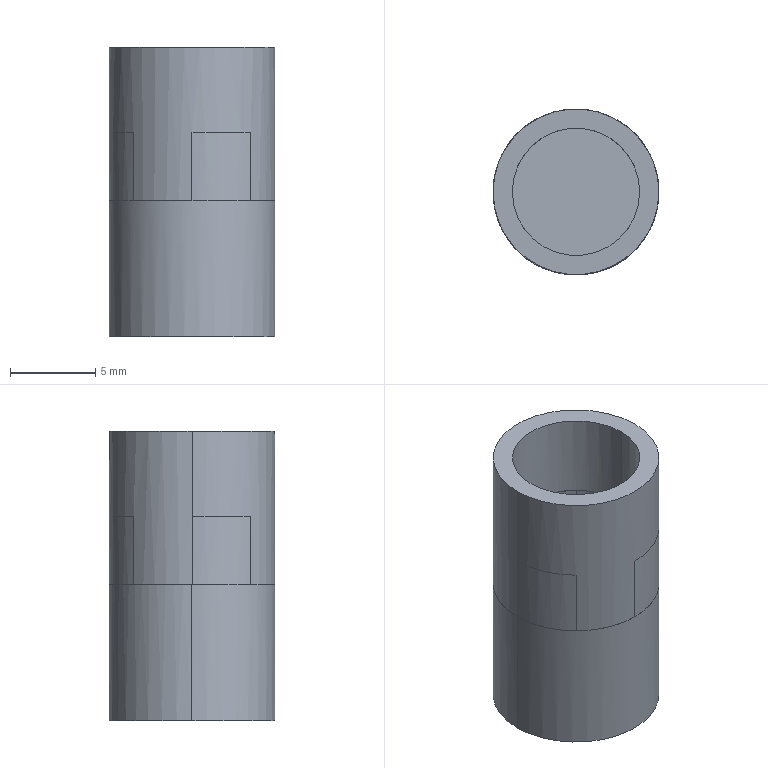Part | SolidWorks | features ICE 3, Extrusion 1 | 2 solids | 47 faces | box 9.746 x 9.746 x 17 mm | volume 515.173 mm3 | plane 28 | cylinder 19 | commonest cylinder face diameters 9.73 x6 7.5 x5 7.516 x4 7.484 x2 9.746 x2
STEP:
#1=CARTESIAN_POINT('',(-3.75,0.007782,-4.));
#2=VERTEX_POINT('',#1);
#3=CARTESIAN_POINT('',(3.75,0.007782,-4.));
#4=VERTEX_POINT('',#3);
#5=CARTESIAN_POINT('',(0.000001501,0.007782,-4.));
#6=DIRECTION('',(0.,0.,1.));
#7=DIRECTION('',(1.,0.,0.));
#8=AXIS2_PLACEMENT_3D('',#5,#6,#7);
#9=CIRCLE('',#8,3.75);
#10=EDGE_CURVE('',#2,#4,#9,.T.);
#11=ORIENTED_EDGE('',*,*,#10,.F.);
#12=CARTESIAN_POINT('',(-3.75,0.007782,4.));
#13=VERTEX_POINT('',#12);
#14=CARTESIAN_POINT('',(-3.75,0.007782,-4.));
#15=DIRECTION('',(0.,0.,1.));
#16=VECTOR('',#15,1000.);
#17=LINE('',#14,#16);
#18=EDGE_CURVE('',#2,#13,#17,.T.);
#19=ORIENTED_EDGE('',*,*,#18,.T.);
#20=CARTESIAN_POINT('',(3.75,0.007782,4.));
#21=VERTEX_POINT('',#20);
#22=CARTESIAN_POINT('',(0.000001501,0.007782,4.));
#23=DIRECTION('',(0.,0.,1.));
#24=DIRECTION('',(1.,0.,0.));
#25=AXIS2_PLACEMENT_3D('',#22,#23,#24);
#26=CIRCLE('',#25,3.75);
#27=EDGE_CURVE('',#13,#21,#26,.T.);
#28=ORIENTED_EDGE('',*,*,#27,.T.);
#29=CARTESIAN_POINT('',(3.75,0.007782,-4.));
#30=DIRECTION('',(0.,0.,1.));
#31=VECTOR('',#30,1000.);
#32=LINE('',#29,#31);
#33=EDGE_CURVE('',#4,#21,#32,.T.);
#34=ORIENTED_EDGE('',*,*,#33,.F.);
#35=EDGE_LOOP('',(#11,#19,#28,#34));
#36=FACE_OUTER_BOUND('',#35,.T.);
#37=CARTESIAN_POINT('',(0.000001501,0.007782,-4.));
#38=DIRECTION('',(0.,0.,1.));
#39=DIRECTION('',(1.,0.,0.));
#40=AXIS2_PLACEMENT_3D('',#37,#38,#39);
#41=CYLINDRICAL_SURFACE('',#40,3.75);
#42=ADVANCED_FACE('',(#36),#41,.F.);
#43=CARTESIAN_POINT('',(4.873,0.007782,-4.));
#44=VERTEX_POINT('',#43);
#45=CARTESIAN_POINT('',(-4.873,0.007782,-4.));
#46=VERTEX_POINT('',#45);
#47=CARTESIAN_POINT('',(0.000001501,0.007782,-4.));
#48=DIRECTION('',(0.,0.,1.));
#49=DIRECTION('',(1.,0.,0.));
#50=AXIS2_PLACEMENT_3D('',#47,#48,#49);
#51=CIRCLE('',#50,4.873);
#52=EDGE_CURVE('',#44,#46,#51,.T.);
#53=ORIENTED_EDGE('',*,*,#52,.T.);
#54=CARTESIAN_POINT('',(-4.873,0.007782,4.));
#55=VERTEX_POINT('',#54);
#56=CARTESIAN_POINT('',(-4.873,0.007782,-4.));
#57=DIRECTION('',(0.,0.,1.));
#58=VECTOR('',#57,1000.);
#59=LINE('',#56,#58);
#60=EDGE_CURVE('',#46,#55,#59,.T.);
#61=ORIENTED_EDGE('',*,*,#60,.T.);
#62=CARTESIAN_POINT('',(4.873,0.007782,4.));
#63=VERTEX_POINT('',#62);
#64=CARTESIAN_POINT('',(0.000001501,0.007782,4.));
#65=DIRECTION('',(0.,0.,1.));
#66=DIRECTION('',(1.,0.,0.));
#67=AXIS2_PLACEMENT_3D('',#64,#65,#66);
#68=CIRCLE('',#67,4.873);
#69=EDGE_CURVE('',#63,#55,#68,.T.);
#70=ORIENTED_EDGE('',*,*,#69,.F.);
#71=CARTESIAN_POINT('',(4.873,0.007782,-4.));
#72=DIRECTION('',(0.,0.,1.));
#73=VECTOR('',#72,1000.);
#74=LINE('',#71,#73);
#75=EDGE_CURVE('',#44,#63,#74,.T.);
#76=ORIENTED_EDGE('',*,*,#75,.F.);
#77=EDGE_LOOP('',(#53,#61,#70,#76));
#78=FACE_OUTER_BOUND('',#77,.T.);
#79=CARTESIAN_POINT('',(0.000001501,0.007782,-4.));
#80=DIRECTION('',(0.,0.,1.));
#81=DIRECTION('',(1.,0.,0.));
#82=AXIS2_PLACEMENT_3D('',#79,#80,#81);
#83=CYLINDRICAL_SURFACE('',#82,4.873);
#84=ADVANCED_FACE('',(#78),#83,.T.);
#85=CARTESIAN_POINT('',(3.758,0.,4.));
#86=VERTEX_POINT('',#85);
#87=CARTESIAN_POINT('',(4.865,0.,4.));
#88=VERTEX_POINT('',#87);
#89=CARTESIAN_POINT('',(3.758,0.,4.));
#90=DIRECTION('',(1.,0.,0.));
#91=VECTOR('',#90,1000.);
#92=LINE('',#89,#91);
#93=EDGE_CURVE('',#86,#88,#92,.T.);
#94=ORIENTED_EDGE('',*,*,#93,.F.);
#95=CARTESIAN_POINT('',(2.656,2.655,4.));
#96=VERTEX_POINT('',#95);
#97=CARTESIAN_POINT('',(0.007782,-0.000001501,4.));
#98=DIRECTION('',(0.,0.,1.));
#99=DIRECTION('',(1.,0.,0.));
#100=AXIS2_PLACEMENT_3D('',#97,#98,#99);
#101=CIRCLE('',#100,3.75);
#102=EDGE_CURVE('',#86,#96,#101,.T.);
#103=ORIENTED_EDGE('',*,*,#102,.T.);
#104=CARTESIAN_POINT('',(0.000001501,0.007782,4.));
#105=DIRECTION('',(0.,0.,1.));
#106=DIRECTION('',(1.,0.,0.));
#107=AXIS2_PLACEMENT_3D('',#104,#105,#106);
#108=CIRCLE('',#107,3.75);
#109=EDGE_CURVE('',#21,#96,#108,.T.);
#110=ORIENTED_EDGE('',*,*,#109,.F.);
#111=ORIENTED_EDGE('',*,*,#27,.F.);
#112=CARTESIAN_POINT('',(-2.656,2.656,4.));
#113=VERTEX_POINT('',#112);
#114=CARTESIAN_POINT('',(0.000001501,0.007782,4.));
#115=DIRECTION('',(0.,0.,1.));
#116=DIRECTION('',(1.,0.,0.));
#117=AXIS2_PLACEMENT_3D('',#114,#115,#116);
#118=CIRCLE('',#117,3.75);
#119=EDGE_CURVE('',#113,#13,#118,.T.);
#120=ORIENTED_EDGE('',*,*,#119,.F.);
#121=CARTESIAN_POINT('',(-3.44,3.44,4.));
#122=VERTEX_POINT('',#121);
#123=CARTESIAN_POINT('',(-2.656,2.656,4.));
#124=DIRECTION('',(0.7071,-0.7071,0.));
#125=VECTOR('',#124,1000.);
#126=LINE('',#123,#125);
#127=EDGE_CURVE('',#122,#113,#126,.T.);
#128=ORIENTED_EDGE('',*,*,#127,.F.);
#129=CARTESIAN_POINT('',(0.,4.865,4.));
#130=VERTEX_POINT('',#129);
#131=CARTESIAN_POINT('',(0.,0.,4.));
#132=DIRECTION('',(0.,0.,1.));
#133=DIRECTION('',(1.,0.,0.));
#134=AXIS2_PLACEMENT_3D('',#131,#132,#133);
#135=CIRCLE('',#134,4.865);
#136=EDGE_CURVE('',#130,#122,#135,.T.);
#137=ORIENTED_EDGE('',*,*,#136,.F.);
#138=CARTESIAN_POINT('',(0.,3.758,4.));
#139=VERTEX_POINT('',#138);
#140=CARTESIAN_POINT('',(0.,3.758,4.));
#141=DIRECTION('',(0.,1.,0.));
#142=VECTOR('',#141,1000.);
#143=LINE('',#140,#142);
#144=EDGE_CURVE('',#139,#130,#143,.T.);
#145=ORIENTED_EDGE('',*,*,#144,.F.);
#146=CARTESIAN_POINT('',(2.656,2.656,4.));
#147=VERTEX_POINT('',#146);
#148=CARTESIAN_POINT('',(0.000001501,0.007782,4.));
#149=DIRECTION('',(0.,0.,1.));
#150=DIRECTION('',(1.,0.,0.));
#151=AXIS2_PLACEMENT_3D('',#148,#149,#150);
#152=CIRCLE('',#151,3.75);
#153=EDGE_CURVE('',#147,#139,#152,.T.);
#154=ORIENTED_EDGE('',*,*,#153,.F.);
#155=CARTESIAN_POINT('',(3.44,3.44,4.));
#156=VERTEX_POINT('',#155);
#157=CARTESIAN_POINT('',(2.656,2.656,4.));
#158=DIRECTION('',(-0.7071,-0.7071,0.));
#159=VECTOR('',#158,1000.);
#160=LINE('',#157,#159);
#161=EDGE_CURVE('',#156,#147,#160,.T.);
#162=ORIENTED_EDGE('',*,*,#161,.F.);
#163=CARTESIAN_POINT('',(0.,0.,4.));
#164=DIRECTION('',(0.,0.,1.));
#165=DIRECTION('',(1.,0.,0.));
#166=AXIS2_PLACEMENT_3D('',#163,#164,#165);
#167=CIRCLE('',#166,4.865);
#168=EDGE_CURVE('',#88,#156,#167,.T.);
#169=ORIENTED_EDGE('',*,*,#168,.F.);
#170=EDGE_LOOP('',(#94,#103,#110,#111,#120,#128,#137,#145,#154,#162,#169));
#171=FACE_BOUND('',#170,.T.);
#172=CARTESIAN_POINT('',(0.,-3.758,4.));
#173=VERTEX_POINT('',#172);
#174=CARTESIAN_POINT('',(0.,-4.865,4.));
#175=VERTEX_POINT('',#174);
#176=CARTESIAN_POINT('',(0.,-3.758,4.));
#177=DIRECTION('',(0.,-1.,0.));
#178=VECTOR('',#177,1000.);
#179=LINE('',#176,#178);
#180=EDGE_CURVE('',#173,#175,#179,.T.);
#181=ORIENTED_EDGE('',*,*,#180,.F.);
#182=CARTESIAN_POINT('',(2.656,-2.656,4.));
#183=VERTEX_POINT('',#182);
#184=CARTESIAN_POINT('',(-0.000001501,-0.007782,4.));
#185=DIRECTION('',(0.,0.,-1.));
#186=DIRECTION('',(1.,0.,0.));
#187=AXIS2_PLACEMENT_3D('',#184,#185,#186);
#188=CIRCLE('',#187,3.75);
#189=EDGE_CURVE('',#183,#173,#188,.T.);
#190=ORIENTED_EDGE('',*,*,#189,.F.);
#191=CARTESIAN_POINT('',(3.44,-3.44,4.));
#192=VERTEX_POINT('',#191);
#193=CARTESIAN_POINT('',(2.656,-2.656,4.));
#194=DIRECTION('',(-0.7071,0.7071,0.));
#195=VECTOR('',#194,1000.);
#196=LINE('',#193,#195);
#197=EDGE_CURVE('',#192,#183,#196,.T.);
#198=ORIENTED_EDGE('',*,*,#197,.F.);
#199=CARTESIAN_POINT('',(0.,0.,4.));
#200=DIRECTION('',(0.,0.,1.));
#201=DIRECTION('',(1.,0.,0.));
#202=AXIS2_PLACEMENT_3D('',#199,#200,#201);
#203=CIRCLE('',#202,4.865);
#204=EDGE_CURVE('',#175,#192,#203,.T.);
#205=ORIENTED_EDGE('',*,*,#204,.F.);
#206=CARTESIAN_POINT('',(0.000001501,0.007782,4.));
#207=DIRECTION('',(0.,0.,1.));
#208=DIRECTION('',(1.,0.,0.));
#209=AXIS2_PLACEMENT_3D('',#206,#207,#208);
#210=CIRCLE('',#209,4.873);
#211=EDGE_CURVE('',#175,#63,#210,.T.);
#212=ORIENTED_EDGE('',*,*,#211,.T.);
#213=ORIENTED_EDGE('',*,*,#69,.T.);
#214=CARTESIAN_POINT('',(0.000001501,0.007782,4.));
#215=DIRECTION('',(0.,0.,1.));
#216=DIRECTION('',(1.,0.,0.));
#217=AXIS2_PLACEMENT_3D('',#214,#215,#216);
#218=CIRCLE('',#217,4.873);
#219=EDGE_CURVE('',#55,#175,#218,.T.);
#220=ORIENTED_EDGE('',*,*,#219,.T.);
#221=EDGE_LOOP('',(#181,#190,#198,#205,#212,#213,#220));
#222=FACE_OUTER_BOUND('',#221,.T.);
#223=CARTESIAN_POINT('',(-3.758,0.,4.));
#224=VERTEX_POINT('',#223);
#225=CARTESIAN_POINT('',(-4.865,0.,4.));
#226=VERTEX_POINT('',#225);
#227=CARTESIAN_POINT('',(-3.758,0.,4.));
#228=DIRECTION('',(-1.,0.,0.));
#229=VECTOR('',#228,1000.);
#230=LINE('',#227,#229);
#231=EDGE_CURVE('',#224,#226,#230,.T.);
#232=ORIENTED_EDGE('',*,*,#231,.F.);
#233=CARTESIAN_POINT('',(-2.656,-2.656,4.));
#234=VERTEX_POINT('',#233);
#235=CARTESIAN_POINT('',(-0.007782,0.000001501,4.));
#236=DIRECTION('',(0.,0.,-1.));
#237=DIRECTION('',(1.,0.,0.));
#238=AXIS2_PLACEMENT_3D('',#235,#236,#237);
#239=CIRCLE('',#238,3.75);
#240=EDGE_CURVE('',#234,#224,#239,.T.);
#241=ORIENTED_EDGE('',*,*,#240,.F.);
#242=CARTESIAN_POINT('',(-3.44,-3.44,4.));
#243=VERTEX_POINT('',#242);
#244=CARTESIAN_POINT('',(-2.656,-2.656,4.));
#245=DIRECTION('',(0.7071,0.7071,0.));
#246=VECTOR('',#245,1000.);
#247=LINE('',#244,#246);
#248=EDGE_CURVE('',#243,#234,#247,.T.);
#249=ORIENTED_EDGE('',*,*,#248,.F.);
#250=CARTESIAN_POINT('',(0.,0.,4.));
#251=DIRECTION('',(0.,0.,1.));
#252=DIRECTION('',(1.,0.,0.));
#253=AXIS2_PLACEMENT_3D('',#250,#251,#252);
#254=CIRCLE('',#253,4.865);
#255=EDGE_CURVE('',#226,#243,#254,.T.);
#256=ORIENTED_EDGE('',*,*,#255,.F.);
#257=EDGE_LOOP('',(#232,#241,#249,#256));
#258=FACE_BOUND('',#257,.T.);
#259=CARTESIAN_POINT('',(0.000001501,0.007782,4.));
#260=DIRECTION('',(0.,0.,1.));
#261=DIRECTION('',(1.,0.,0.));
#262=AXIS2_PLACEMENT_3D('',#259,#260,#261);
#263=PLANE('',#262);
#264=ADVANCED_FACE('',(#171,#222,#258),#263,.T.);
#265=ORIENTED_EDGE('',*,*,#60,.F.);
#266=CARTESIAN_POINT('',(0.000001501,0.007782,-4.));
#267=DIRECTION('',(0.,0.,1.));
#268=DIRECTION('',(1.,0.,0.));
#269=AXIS2_PLACEMENT_3D('',#266,#267,#268);
#270=CIRCLE('',#269,4.873);
#271=EDGE_CURVE('',#46,#44,#270,.T.);
#272=ORIENTED_EDGE('',*,*,#271,.T.);
#273=ORIENTED_EDGE('',*,*,#75,.T.);
#274=ORIENTED_EDGE('',*,*,#211,.F.);
#275=ORIENTED_EDGE('',*,*,#219,.F.);
#276=EDGE_LOOP('',(#265,#272,#273,#274,#275));
#277=FACE_OUTER_BOUND('',#276,.T.);
#278=CARTESIAN_POINT('',(0.000001501,0.007782,-4.));
#279=DIRECTION('',(0.,0.,1.));
#280=DIRECTION('',(1.,0.,0.));
#281=AXIS2_PLACEMENT_3D('',#278,#279,#280);
#282=CYLINDRICAL_SURFACE('',#281,4.873);
#283=ADVANCED_FACE('',(#277),#282,.T.);
#284=CARTESIAN_POINT('',(0.000001501,0.007782,-4.));
#285=DIRECTION('',(0.,0.,1.));
#286=DIRECTION('',(1.,0.,0.));
#287=AXIS2_PLACEMENT_3D('',#284,#285,#286);
#288=CIRCLE('',#287,3.75);
#289=EDGE_CURVE('',#4,#2,#288,.T.);
#290=ORIENTED_EDGE('',*,*,#289,.T.);
#291=ORIENTED_EDGE('',*,*,#10,.T.);
#292=EDGE_LOOP('',(#290,#291));
#293=FACE_BOUND('',#292,.T.);
#294=ORIENTED_EDGE('',*,*,#52,.F.);
#295=ORIENTED_EDGE('',*,*,#271,.F.);
#296=EDGE_LOOP('',(#294,#295));
#297=FACE_OUTER_BOUND('',#296,.T.);
#298=CARTESIAN_POINT('',(0.000001501,0.007782,-4.));
#299=DIRECTION('',(0.,0.,1.));
#300=DIRECTION('',(1.,0.,0.));
#301=AXIS2_PLACEMENT_3D('',#298,#299,#300);
#302=PLANE('',#301);
#303=ADVANCED_FACE('',(#293,#297),#302,.F.);
#304=ORIENTED_EDGE('',*,*,#18,.F.);
#305=ORIENTED_EDGE('',*,*,#289,.F.);
#306=ORIENTED_EDGE('',*,*,#33,.T.);
#307=ORIENTED_EDGE('',*,*,#109,.T.);
#308=CARTESIAN_POINT('',(0.007782,-0.000001501,4.));
#309=DIRECTION('',(0.,0.,-1.));
#310=DIRECTION('',(1.,0.,0.));
#311=AXIS2_PLACEMENT_3D('',#308,#309,#310);
#312=CIRCLE('',#311,3.75);
#313=EDGE_CURVE('',#147,#96,#312,.T.);
#314=ORIENTED_EDGE('',*,*,#313,.F.);
#315=ORIENTED_EDGE('',*,*,#153,.T.);
#316=CARTESIAN_POINT('',(0.,3.758,8.));
#317=VERTEX_POINT('',#316);
#318=CARTESIAN_POINT('',(0.,3.758,8.));
#319=DIRECTION('',(0.,0.,-1.));
#320=VECTOR('',#319,1000.);
#321=LINE('',#318,#320);
#322=EDGE_CURVE('',#317,#139,#321,.T.);
#323=ORIENTED_EDGE('',*,*,#322,.F.);
#324=CARTESIAN_POINT('',(-2.656,2.656,8.));
#325=VERTEX_POINT('',#324);
#326=CARTESIAN_POINT('',(0.000001501,0.007782,8.));
#327=DIRECTION('',(0.,0.,-1.));
#328=DIRECTION('',(1.,0.,0.));
#329=AXIS2_PLACEMENT_3D('',#326,#327,#328);
#330=CIRCLE('',#329,3.75);
#331=EDGE_CURVE('',#325,#317,#330,.T.);
#332=ORIENTED_EDGE('',*,*,#331,.F.);
#333=CARTESIAN_POINT('',(-2.656,2.656,8.));
#334=DIRECTION('',(0.,0.,-1.));
#335=VECTOR('',#334,1000.);
#336=LINE('',#333,#335);
#337=EDGE_CURVE('',#325,#113,#336,.T.);
#338=ORIENTED_EDGE('',*,*,#337,.T.);
#339=ORIENTED_EDGE('',*,*,#119,.T.);
#340=EDGE_LOOP('',(#304,#305,#306,#307,#314,#315,#323,#332,#338,#339));
#341=FACE_OUTER_BOUND('',#340,.T.);
#342=CARTESIAN_POINT('',(0.000001501,0.007782,-4.));
#343=DIRECTION('',(0.,0.,1.));
#344=DIRECTION('',(1.,0.,0.));
#345=AXIS2_PLACEMENT_3D('',#342,#343,#344);
#346=CYLINDRICAL_SURFACE('',#345,3.75);
#347=ADVANCED_FACE('',(#341),#346,.F.);
#348=ORIENTED_EDGE('',*,*,#144,.T.);
#349=CARTESIAN_POINT('',(0.,4.865,8.));
#350=VERTEX_POINT('',#349);
#351=CARTESIAN_POINT('',(0.,4.865,8.));
#352=DIRECTION('',(0.,0.,-1.));
#353=VECTOR('',#352,1000.);
#354=LINE('',#351,#353);
#355=EDGE_CURVE('',#350,#130,#354,.T.);
#356=ORIENTED_EDGE('',*,*,#355,.F.);
#357=CARTESIAN_POINT('',(0.,3.758,8.));
#358=DIRECTION('',(0.,1.,0.));
#359=VECTOR('',#358,1000.);
#360=LINE('',#357,#359);
#361=EDGE_CURVE('',#317,#350,#360,.T.);
#362=ORIENTED_EDGE('',*,*,#361,.F.);
#363=ORIENTED_EDGE('',*,*,#322,.T.);
#364=EDGE_LOOP('',(#348,#356,#362,#363));
#365=FACE_OUTER_BOUND('',#364,.T.);
#366=CARTESIAN_POINT('',(0.,3.758,8.));
#367=DIRECTION('',(-1.,0.,0.));
#368=DIRECTION('',(0.,0.,1.));
#369=AXIS2_PLACEMENT_3D('',#366,#367,#368);
#370=PLANE('',#369);
#371=ADVANCED_FACE('',(#365),#370,.F.);
#372=ORIENTED_EDGE('',*,*,#136,.T.);
#373=CARTESIAN_POINT('',(-3.44,3.44,8.));
#374=VERTEX_POINT('',#373);
#375=CARTESIAN_POINT('',(-3.44,3.44,8.));
#376=DIRECTION('',(0.,0.,-1.));
#377=VECTOR('',#376,1000.);
#378=LINE('',#375,#377);
#379=EDGE_CURVE('',#374,#122,#378,.T.);
#380=ORIENTED_EDGE('',*,*,#379,.F.);
#381=CARTESIAN_POINT('',(0.,0.,8.));
#382=DIRECTION('',(0.,0.,1.));
#383=DIRECTION('',(1.,0.,0.));
#384=AXIS2_PLACEMENT_3D('',#381,#382,#383);
#385=CIRCLE('',#384,4.865);
#386=EDGE_CURVE('',#350,#374,#385,.T.);
#387=ORIENTED_EDGE('',*,*,#386,.F.);
#388=ORIENTED_EDGE('',*,*,#355,.T.);
#389=EDGE_LOOP('',(#372,#380,#387,#388));
#390=FACE_OUTER_BOUND('',#389,.T.);
#391=CARTESIAN_POINT('',(0.,0.,8.));
#392=DIRECTION('',(0.,0.,-1.));
#393=DIRECTION('',(-1.,0.,0.));
#394=AXIS2_PLACEMENT_3D('',#391,#392,#393);
#395=CYLINDRICAL_SURFACE('',#394,4.865);
#396=ADVANCED_FACE('',(#390),#395,.T.);
#397=ORIENTED_EDGE('',*,*,#127,.T.);
#398=ORIENTED_EDGE('',*,*,#337,.F.);
#399=CARTESIAN_POINT('',(-2.656,2.656,8.));
#400=DIRECTION('',(0.7071,-0.7071,0.));
#401=VECTOR('',#400,1000.);
#402=LINE('',#399,#401);
#403=EDGE_CURVE('',#374,#325,#402,.T.);
#404=ORIENTED_EDGE('',*,*,#403,.F.);
#405=ORIENTED_EDGE('',*,*,#379,.T.);
#406=EDGE_LOOP('',(#397,#398,#404,#405));
#407=FACE_OUTER_BOUND('',#406,.T.);
#408=CARTESIAN_POINT('',(-2.656,2.656,8.));
#409=DIRECTION('',(0.7071,0.7071,0.));
#410=DIRECTION('',(-0.7071,0.7071,0.));
#411=AXIS2_PLACEMENT_3D('',#408,#409,#410);
#412=PLANE('',#411);
#413=ADVANCED_FACE('',(#407),#412,.F.);
#414=ORIENTED_EDGE('',*,*,#331,.T.);
#415=ORIENTED_EDGE('',*,*,#361,.T.);
#416=ORIENTED_EDGE('',*,*,#386,.T.);
#417=ORIENTED_EDGE('',*,*,#403,.T.);
#418=EDGE_LOOP('',(#414,#415,#416,#417));
#419=FACE_OUTER_BOUND('',#418,.T.);
#420=CARTESIAN_POINT('',(0.000001501,0.007782,8.));
#421=DIRECTION('',(0.,0.,1.));
#422=DIRECTION('',(1.,0.,0.));
#423=AXIS2_PLACEMENT_3D('',#420,#421,#422);
#424=PLANE('',#423);
#425=ADVANCED_FACE('',(#419),#424,.T.);
#426=ORIENTED_EDGE('',*,*,#313,.T.);
#427=ORIENTED_EDGE('',*,*,#102,.F.);
#428=CARTESIAN_POINT('',(3.758,0.,8.));
#429=VERTEX_POINT('',#428);
#430=CARTESIAN_POINT('',(3.758,0.,8.));
#431=DIRECTION('',(0.,0.,-1.));
#432=VECTOR('',#431,1000.);
#433=LINE('',#430,#432);
#434=EDGE_CURVE('',#429,#86,#433,.T.);
#435=ORIENTED_EDGE('',*,*,#434,.F.);
#436=CARTESIAN_POINT('',(2.656,2.656,8.));
#437=VERTEX_POINT('',#436);
#438=CARTESIAN_POINT('',(0.007782,-0.000001501,8.));
#439=DIRECTION('',(0.,0.,-1.));
#440=DIRECTION('',(1.,0.,0.));
#441=AXIS2_PLACEMENT_3D('',#438,#439,#440);
#442=CIRCLE('',#441,3.75);
#443=EDGE_CURVE('',#437,#429,#442,.T.);
#444=ORIENTED_EDGE('',*,*,#443,.F.);
#445=CARTESIAN_POINT('',(2.656,2.656,8.));
#446=DIRECTION('',(0.,0.,-1.));
#447=VECTOR('',#446,1000.);
#448=LINE('',#445,#447);
#449=EDGE_CURVE('',#437,#147,#448,.T.);
#450=ORIENTED_EDGE('',*,*,#449,.T.);
#451=EDGE_LOOP('',(#426,#427,#435,#444,#450));
#452=FACE_OUTER_BOUND('',#451,.T.);
#453=CARTESIAN_POINT('',(0.007782,-0.000001501,8.));
#454=DIRECTION('',(0.,0.,-1.));
#455=DIRECTION('',(-1.,0.,0.));
#456=AXIS2_PLACEMENT_3D('',#453,#454,#455);
#457=CYLINDRICAL_SURFACE('',#456,3.75);
#458=ADVANCED_FACE('',(#452),#457,.F.);
#459=ORIENTED_EDGE('',*,*,#93,.T.);
#460=CARTESIAN_POINT('',(4.865,0.,8.));
#461=VERTEX_POINT('',#460);
#462=CARTESIAN_POINT('',(4.865,0.,8.));
#463=DIRECTION('',(0.,0.,-1.));
#464=VECTOR('',#463,1000.);
#465=LINE('',#462,#464);
#466=EDGE_CURVE('',#461,#88,#465,.T.);
#467=ORIENTED_EDGE('',*,*,#466,.F.);
#468=CARTESIAN_POINT('',(3.758,0.,8.));
#469=DIRECTION('',(1.,0.,0.));
#470=VECTOR('',#469,1000.);
#471=LINE('',#468,#470);
#472=EDGE_CURVE('',#429,#461,#471,.T.);
#473=ORIENTED_EDGE('',*,*,#472,.F.);
#474=ORIENTED_EDGE('',*,*,#434,.T.);
#475=EDGE_LOOP('',(#459,#467,#473,#474));
#476=FACE_OUTER_BOUND('',#475,.T.);
#477=CARTESIAN_POINT('',(3.758,0.,8.));
#478=DIRECTION('',(0.,1.,0.));
#479=DIRECTION('',(-1.,0.,0.));
#480=AXIS2_PLACEMENT_3D('',#477,#478,#479);
#481=PLANE('',#480);
#482=ADVANCED_FACE('',(#476),#481,.F.);
#483=ORIENTED_EDGE('',*,*,#168,.T.);
#484=CARTESIAN_POINT('',(3.44,3.44,8.));
#485=VERTEX_POINT('',#484);
#486=CARTESIAN_POINT('',(3.44,3.44,8.));
#487=DIRECTION('',(0.,0.,-1.));
#488=VECTOR('',#487,1000.);
#489=LINE('',#486,#488);
#490=EDGE_CURVE('',#485,#156,#489,.T.);
#491=ORIENTED_EDGE('',*,*,#490,.F.);
#492=CARTESIAN_POINT('',(0.,0.,8.));
#493=DIRECTION('',(0.,0.,1.));
#494=DIRECTION('',(1.,0.,0.));
#495=AXIS2_PLACEMENT_3D('',#492,#493,#494);
#496=CIRCLE('',#495,4.865);
#497=EDGE_CURVE('',#461,#485,#496,.T.);
#498=ORIENTED_EDGE('',*,*,#497,.F.);
#499=ORIENTED_EDGE('',*,*,#466,.T.);
#500=EDGE_LOOP('',(#483,#491,#498,#499));
#501=FACE_OUTER_BOUND('',#500,.T.);
#502=CARTESIAN_POINT('',(0.,0.,8.));
#503=DIRECTION('',(0.,0.,-1.));
#504=DIRECTION('',(-1.,0.,0.));
#505=AXIS2_PLACEMENT_3D('',#502,#503,#504);
#506=CYLINDRICAL_SURFACE('',#505,4.865);
#507=ADVANCED_FACE('',(#501),#506,.T.);
#508=ORIENTED_EDGE('',*,*,#161,.T.);
#509=ORIENTED_EDGE('',*,*,#449,.F.);
#510=CARTESIAN_POINT('',(2.656,2.656,8.));
#511=DIRECTION('',(-0.7071,-0.7071,0.));
#512=VECTOR('',#511,1000.);
#513=LINE('',#510,#512);
#514=EDGE_CURVE('',#485,#437,#513,.T.);
#515=ORIENTED_EDGE('',*,*,#514,.F.);
#516=ORIENTED_EDGE('',*,*,#490,.T.);
#517=EDGE_LOOP('',(#508,#509,#515,#516));
#518=FACE_OUTER_BOUND('',#517,.T.);
#519=CARTESIAN_POINT('',(2.656,2.656,8.));
#520=DIRECTION('',(0.7071,-0.7071,0.));
#521=DIRECTION('',(0.7071,0.7071,0.));
#522=AXIS2_PLACEMENT_3D('',#519,#520,#521);
#523=PLANE('',#522);
#524=ADVANCED_FACE('',(#518),#523,.F.);
#525=ORIENTED_EDGE('',*,*,#443,.T.);
#526=ORIENTED_EDGE('',*,*,#472,.T.);
#527=ORIENTED_EDGE('',*,*,#497,.T.);
#528=ORIENTED_EDGE('',*,*,#514,.T.);
#529=EDGE_LOOP('',(#525,#526,#527,#528));
#530=FACE_OUTER_BOUND('',#529,.T.);
#531=CARTESIAN_POINT('',(0.007782,-0.000001501,8.));
#532=DIRECTION('',(0.,0.,1.));
#533=DIRECTION('',(1.,0.,0.));
#534=AXIS2_PLACEMENT_3D('',#531,#532,#533);
#535=PLANE('',#534);
#536=ADVANCED_FACE('',(#530),#535,.T.);
#537=ORIENTED_EDGE('',*,*,#189,.T.);
#538=CARTESIAN_POINT('',(0.,-3.758,8.));
#539=VERTEX_POINT('',#538);
#540=CARTESIAN_POINT('',(0.,-3.758,8.));
#541=DIRECTION('',(0.,0.,-1.));
#542=VECTOR('',#541,1000.);
#543=LINE('',#540,#542);
#544=EDGE_CURVE('',#539,#173,#543,.T.);
#545=ORIENTED_EDGE('',*,*,#544,.F.);
#546=CARTESIAN_POINT('',(2.656,-2.656,8.));
#547=VERTEX_POINT('',#546);
#548=CARTESIAN_POINT('',(-0.000001501,-0.007782,8.));
#549=DIRECTION('',(0.,0.,-1.));
#550=DIRECTION('',(1.,0.,0.));
#551=AXIS2_PLACEMENT_3D('',#548,#549,#550);
#552=CIRCLE('',#551,3.75);
#553=EDGE_CURVE('',#547,#539,#552,.T.);
#554=ORIENTED_EDGE('',*,*,#553,.F.);
#555=CARTESIAN_POINT('',(2.656,-2.656,8.));
#556=DIRECTION('',(0.,0.,-1.));
#557=VECTOR('',#556,1000.);
#558=LINE('',#555,#557);
#559=EDGE_CURVE('',#547,#183,#558,.T.);
#560=ORIENTED_EDGE('',*,*,#559,.T.);
#561=EDGE_LOOP('',(#537,#545,#554,#560));
#562=FACE_OUTER_BOUND('',#561,.T.);
#563=CARTESIAN_POINT('',(-0.000001501,-0.007782,8.));
#564=DIRECTION('',(0.,0.,-1.));
#565=DIRECTION('',(-1.,0.,0.));
#566=AXIS2_PLACEMENT_3D('',#563,#564,#565);
#567=CYLINDRICAL_SURFACE('',#566,3.75);
#568=ADVANCED_FACE('',(#562),#567,.F.);
#569=ORIENTED_EDGE('',*,*,#180,.T.);
#570=CARTESIAN_POINT('',(0.,-4.865,8.));
#571=VERTEX_POINT('',#570);
#572=CARTESIAN_POINT('',(0.,-4.865,8.));
#573=DIRECTION('',(0.,0.,-1.));
#574=VECTOR('',#573,1000.);
#575=LINE('',#572,#574);
#576=EDGE_CURVE('',#571,#175,#575,.T.);
#577=ORIENTED_EDGE('',*,*,#576,.F.);
#578=CARTESIAN_POINT('',(0.,-3.758,8.));
#579=DIRECTION('',(0.,-1.,0.));
#580=VECTOR('',#579,1000.);
#581=LINE('',#578,#580);
#582=EDGE_CURVE('',#539,#571,#581,.T.);
#583=ORIENTED_EDGE('',*,*,#582,.F.);
#584=ORIENTED_EDGE('',*,*,#544,.T.);
#585=EDGE_LOOP('',(#569,#577,#583,#584));
#586=FACE_OUTER_BOUND('',#585,.T.);
#587=CARTESIAN_POINT('',(0.,-3.758,8.));
#588=DIRECTION('',(1.,0.,0.));
#589=DIRECTION('',(0.,1.,0.));
#590=AXIS2_PLACEMENT_3D('',#587,#588,#589);
#591=PLANE('',#590);
#592=ADVANCED_FACE('',(#586),#591,.F.);
#593=ORIENTED_EDGE('',*,*,#204,.T.);
#594=CARTESIAN_POINT('',(3.44,-3.44,8.));
#595=VERTEX_POINT('',#594);
#596=CARTESIAN_POINT('',(3.44,-3.44,8.));
#597=DIRECTION('',(0.,0.,-1.));
#598=VECTOR('',#597,1000.);
#599=LINE('',#596,#598);
#600=EDGE_CURVE('',#595,#192,#599,.T.);
#601=ORIENTED_EDGE('',*,*,#600,.F.);
#602=CARTESIAN_POINT('',(0.,0.,8.));
#603=DIRECTION('',(0.,0.,1.));
#604=DIRECTION('',(1.,0.,0.));
#605=AXIS2_PLACEMENT_3D('',#602,#603,#604);
#606=CIRCLE('',#605,4.865);
#607=EDGE_CURVE('',#571,#595,#606,.T.);
#608=ORIENTED_EDGE('',*,*,#607,.F.);
#609=ORIENTED_EDGE('',*,*,#576,.T.);
#610=EDGE_LOOP('',(#593,#601,#608,#609));
#611=FACE_OUTER_BOUND('',#610,.T.);
#612=CARTESIAN_POINT('',(0.,0.,8.));
#613=DIRECTION('',(0.,0.,-1.));
#614=DIRECTION('',(-1.,0.,0.));
#615=AXIS2_PLACEMENT_3D('',#612,#613,#614);
#616=CYLINDRICAL_SURFACE('',#615,4.865);
#617=ADVANCED_FACE('',(#611),#616,.T.);
#618=ORIENTED_EDGE('',*,*,#197,.T.);
#619=ORIENTED_EDGE('',*,*,#559,.F.);
#620=CARTESIAN_POINT('',(2.656,-2.656,8.));
#621=DIRECTION('',(-0.7071,0.7071,0.));
#622=VECTOR('',#621,1000.);
#623=LINE('',#620,#622);
#624=EDGE_CURVE('',#595,#547,#623,.T.);
#625=ORIENTED_EDGE('',*,*,#624,.F.);
#626=ORIENTED_EDGE('',*,*,#600,.T.);
#627=EDGE_LOOP('',(#618,#619,#625,#626));
#628=FACE_OUTER_BOUND('',#627,.T.);
#629=CARTESIAN_POINT('',(2.656,-2.656,8.));
#630=DIRECTION('',(-0.7071,-0.7071,0.));
#631=DIRECTION('',(0.7071,-0.7071,0.));
#632=AXIS2_PLACEMENT_3D('',#629,#630,#631);
#633=PLANE('',#632);
#634=ADVANCED_FACE('',(#628),#633,.F.);
#635=ORIENTED_EDGE('',*,*,#553,.T.);
#636=ORIENTED_EDGE('',*,*,#582,.T.);
#637=ORIENTED_EDGE('',*,*,#607,.T.);
#638=ORIENTED_EDGE('',*,*,#624,.T.);
#639=EDGE_LOOP('',(#635,#636,#637,#638));
#640=FACE_OUTER_BOUND('',#639,.T.);
#641=CARTESIAN_POINT('',(-0.000001501,-0.007782,8.));
#642=DIRECTION('',(0.,0.,1.));
#643=DIRECTION('',(1.,0.,0.));
#644=AXIS2_PLACEMENT_3D('',#641,#642,#643);
#645=PLANE('',#644);
#646=ADVANCED_FACE('',(#640),#645,.T.);
#647=ORIENTED_EDGE('',*,*,#240,.T.);
#648=CARTESIAN_POINT('',(-3.758,0.,8.));
#649=VERTEX_POINT('',#648);
#650=CARTESIAN_POINT('',(-3.758,0.,8.));
#651=DIRECTION('',(0.,0.,-1.));
#652=VECTOR('',#651,1000.);
#653=LINE('',#650,#652);
#654=EDGE_CURVE('',#649,#224,#653,.T.);
#655=ORIENTED_EDGE('',*,*,#654,.F.);
#656=CARTESIAN_POINT('',(-2.656,-2.656,8.));
#657=VERTEX_POINT('',#656);
#658=CARTESIAN_POINT('',(-0.007782,0.000001501,8.));
#659=DIRECTION('',(0.,0.,-1.));
#660=DIRECTION('',(1.,0.,0.));
#661=AXIS2_PLACEMENT_3D('',#658,#659,#660);
#662=CIRCLE('',#661,3.75);
#663=EDGE_CURVE('',#657,#649,#662,.T.);
#664=ORIENTED_EDGE('',*,*,#663,.F.);
#665=CARTESIAN_POINT('',(-2.656,-2.656,8.));
#666=DIRECTION('',(0.,0.,-1.));
#667=VECTOR('',#666,1000.);
#668=LINE('',#665,#667);
#669=EDGE_CURVE('',#657,#234,#668,.T.);
#670=ORIENTED_EDGE('',*,*,#669,.T.);
#671=EDGE_LOOP('',(#647,#655,#664,#670));
#672=FACE_OUTER_BOUND('',#671,.T.);
#673=CARTESIAN_POINT('',(-0.007782,0.000001501,8.));
#674=DIRECTION('',(0.,0.,-1.));
#675=DIRECTION('',(-1.,0.,0.));
#676=AXIS2_PLACEMENT_3D('',#673,#674,#675);
#677=CYLINDRICAL_SURFACE('',#676,3.75);
#678=ADVANCED_FACE('',(#672),#677,.F.);
#679=ORIENTED_EDGE('',*,*,#231,.T.);
#680=CARTESIAN_POINT('',(-4.865,0.,8.));
#681=VERTEX_POINT('',#680);
#682=CARTESIAN_POINT('',(-4.865,0.,8.));
#683=DIRECTION('',(0.,0.,-1.));
#684=VECTOR('',#683,1000.);
#685=LINE('',#682,#684);
#686=EDGE_CURVE('',#681,#226,#685,.T.);
#687=ORIENTED_EDGE('',*,*,#686,.F.);
#688=CARTESIAN_POINT('',(-3.758,0.,8.));
#689=DIRECTION('',(-1.,0.,0.));
#690=VECTOR('',#689,1000.);
#691=LINE('',#688,#690);
#692=EDGE_CURVE('',#649,#681,#691,.T.);
#693=ORIENTED_EDGE('',*,*,#692,.F.);
#694=ORIENTED_EDGE('',*,*,#654,.T.);
#695=EDGE_LOOP('',(#679,#687,#693,#694));
#696=FACE_OUTER_BOUND('',#695,.T.);
#697=CARTESIAN_POINT('',(-3.758,0.,8.));
#698=DIRECTION('',(0.,-1.,0.));
#699=DIRECTION('',(1.,0.,0.));
#700=AXIS2_PLACEMENT_3D('',#697,#698,#699);
#701=PLANE('',#700);
#702=ADVANCED_FACE('',(#696),#701,.F.);
#703=ORIENTED_EDGE('',*,*,#255,.T.);
#704=CARTESIAN_POINT('',(-3.44,-3.44,8.));
#705=VERTEX_POINT('',#704);
#706=CARTESIAN_POINT('',(-3.44,-3.44,8.));
#707=DIRECTION('',(0.,0.,-1.));
#708=VECTOR('',#707,1000.);
#709=LINE('',#706,#708);
#710=EDGE_CURVE('',#705,#243,#709,.T.);
#711=ORIENTED_EDGE('',*,*,#710,.F.);
#712=CARTESIAN_POINT('',(0.,0.,8.));
#713=DIRECTION('',(0.,0.,1.));
#714=DIRECTION('',(1.,0.,0.));
#715=AXIS2_PLACEMENT_3D('',#712,#713,#714);
#716=CIRCLE('',#715,4.865);
#717=EDGE_CURVE('',#681,#705,#716,.T.);
#718=ORIENTED_EDGE('',*,*,#717,.F.);
#719=ORIENTED_EDGE('',*,*,#686,.T.);
#720=EDGE_LOOP('',(#703,#711,#718,#719));
#721=FACE_OUTER_BOUND('',#720,.T.);
#722=CARTESIAN_POINT('',(0.,0.,8.));
#723=DIRECTION('',(0.,0.,-1.));
#724=DIRECTION('',(-1.,0.,0.));
#725=AXIS2_PLACEMENT_3D('',#722,#723,#724);
#726=CYLINDRICAL_SURFACE('',#725,4.865);
#727=ADVANCED_FACE('',(#721),#726,.T.);
#728=ORIENTED_EDGE('',*,*,#248,.T.);
#729=ORIENTED_EDGE('',*,*,#669,.F.);
#730=CARTESIAN_POINT('',(-2.656,-2.656,8.));
#731=DIRECTION('',(0.7071,0.7071,0.));
#732=VECTOR('',#731,1000.);
#733=LINE('',#730,#732);
#734=EDGE_CURVE('',#705,#657,#733,.T.);
#735=ORIENTED_EDGE('',*,*,#734,.F.);
#736=ORIENTED_EDGE('',*,*,#710,.T.);
#737=EDGE_LOOP('',(#728,#729,#735,#736));
#738=FACE_OUTER_BOUND('',#737,.T.);
#739=CARTESIAN_POINT('',(-2.656,-2.656,8.));
#740=DIRECTION('',(-0.7071,0.7071,0.));
#741=DIRECTION('',(-0.7071,-0.7071,0.));
#742=AXIS2_PLACEMENT_3D('',#739,#740,#741);
#743=PLANE('',#742);
#744=ADVANCED_FACE('',(#738),#743,.F.);
#745=ORIENTED_EDGE('',*,*,#663,.T.);
#746=ORIENTED_EDGE('',*,*,#692,.T.);
#747=ORIENTED_EDGE('',*,*,#717,.T.);
#748=ORIENTED_EDGE('',*,*,#734,.T.);
#749=EDGE_LOOP('',(#745,#746,#747,#748));
#750=FACE_OUTER_BOUND('',#749,.T.);
#751=CARTESIAN_POINT('',(-0.007782,0.000001501,8.));
#752=DIRECTION('',(0.,0.,1.));
#753=DIRECTION('',(1.,0.,0.));
#754=AXIS2_PLACEMENT_3D('',#751,#752,#753);
#755=PLANE('',#754);
#756=ADVANCED_FACE('',(#750),#755,.T.);
#757=CLOSED_SHELL('',(#42,#84,#264,#283,#303,#347,#371,#396,#413,#425,#458,#482,#507,#524,#536,#568,#592,#617,#634,#646,#678,#702,#727,#744,#756));
#758=MANIFOLD_SOLID_BREP('',#757);
#759=CARTESIAN_POINT('',(-3.742,0.,13.));
#760=VERTEX_POINT('',#759);
#761=CARTESIAN_POINT('',(3.742,0.,13.));
#762=VERTEX_POINT('',#761);
#763=CARTESIAN_POINT('',(0.,0.,13.));
#764=DIRECTION('',(0.,0.,1.));
#765=DIRECTION('',(1.,0.,0.));
#766=AXIS2_PLACEMENT_3D('',#763,#764,#765);
#767=CIRCLE('',#766,3.742);
#768=EDGE_CURVE('',#760,#762,#767,.T.);
#769=ORIENTED_EDGE('',*,*,#768,.T.);
#770=CARTESIAN_POINT('',(3.742,0.,8.));
#771=VERTEX_POINT('',#770);
#772=CARTESIAN_POINT('',(3.742,0.,13.));
#773=DIRECTION('',(0.,0.,-1.));
#774=VECTOR('',#773,1000.);
#775=LINE('',#772,#774);
#776=EDGE_CURVE('',#762,#771,#775,.T.);
#777=ORIENTED_EDGE('',*,*,#776,.T.);
#778=CARTESIAN_POINT('',(-3.742,0.,8.));
#779=VERTEX_POINT('',#778);
#780=CARTESIAN_POINT('',(0.,0.,8.));
#781=DIRECTION('',(0.,0.,1.));
#782=DIRECTION('',(1.,0.,0.));
#783=AXIS2_PLACEMENT_3D('',#780,#781,#782);
#784=CIRCLE('',#783,3.742);
#785=EDGE_CURVE('',#779,#771,#784,.T.);
#786=ORIENTED_EDGE('',*,*,#785,.F.);
#787=CARTESIAN_POINT('',(-3.742,0.,13.));
#788=DIRECTION('',(0.,0.,-1.));
#789=VECTOR('',#788,1000.);
#790=LINE('',#787,#789);
#791=EDGE_CURVE('',#760,#779,#790,.T.);
#792=ORIENTED_EDGE('',*,*,#791,.F.);
#793=EDGE_LOOP('',(#769,#777,#786,#792));
#794=FACE_OUTER_BOUND('',#793,.T.);
#795=CARTESIAN_POINT('',(0.,0.,13.));
#796=DIRECTION('',(0.,0.,-1.));
#797=DIRECTION('',(-1.,0.,0.));
#798=AXIS2_PLACEMENT_3D('',#795,#796,#797);
#799=CYLINDRICAL_SURFACE('',#798,3.742);
#800=ADVANCED_FACE('',(#794),#799,.F.);
#801=CARTESIAN_POINT('',(4.865,0.,13.));
#802=VERTEX_POINT('',#801);
#803=CARTESIAN_POINT('',(-4.865,0.,13.));
#804=VERTEX_POINT('',#803);
#805=CARTESIAN_POINT('',(0.,0.,13.));
#806=DIRECTION('',(0.,0.,1.));
#807=DIRECTION('',(1.,0.,0.));
#808=AXIS2_PLACEMENT_3D('',#805,#806,#807);
#809=CIRCLE('',#808,4.865);
#810=EDGE_CURVE('',#802,#804,#809,.T.);
#811=ORIENTED_EDGE('',*,*,#810,.F.);
#812=CARTESIAN_POINT('',(4.865,0.,8.));
#813=VERTEX_POINT('',#812);
#814=CARTESIAN_POINT('',(4.865,0.,13.));
#815=DIRECTION('',(0.,0.,-1.));
#816=VECTOR('',#815,1000.);
#817=LINE('',#814,#816);
#818=EDGE_CURVE('',#802,#813,#817,.T.);
#819=ORIENTED_EDGE('',*,*,#818,.T.);
#820=CARTESIAN_POINT('',(3.44,3.44,8.));
#821=VERTEX_POINT('',#820);
#822=CARTESIAN_POINT('',(0.,0.,8.));
#823=DIRECTION('',(0.,0.,1.));
#824=DIRECTION('',(1.,0.,0.));
#825=AXIS2_PLACEMENT_3D('',#822,#823,#824);
#826=CIRCLE('',#825,4.865);
#827=EDGE_CURVE('',#813,#821,#826,.T.);
#828=ORIENTED_EDGE('',*,*,#827,.T.);
#829=CARTESIAN_POINT('',(3.44,3.44,4.));
#830=VERTEX_POINT('',#829);
#831=CARTESIAN_POINT('',(3.44,3.44,4.));
#832=DIRECTION('',(0.,0.,1.));
#833=VECTOR('',#832,1000.);
#834=LINE('',#831,#833);
#835=EDGE_CURVE('',#830,#821,#834,.T.);
#836=ORIENTED_EDGE('',*,*,#835,.F.);
#837=CARTESIAN_POINT('',(0.,4.865,4.));
#838=VERTEX_POINT('',#837);
#839=CARTESIAN_POINT('',(0.,0.,4.));
#840=DIRECTION('',(0.,0.,-1.));
#841=DIRECTION('',(-1.,0.,0.));
#842=AXIS2_PLACEMENT_3D('',#839,#840,#841);
#843=CIRCLE('',#842,4.865);
#844=EDGE_CURVE('',#838,#830,#843,.T.);
#845=ORIENTED_EDGE('',*,*,#844,.F.);
#846=CARTESIAN_POINT('',(0.,4.865,8.));
#847=VERTEX_POINT('',#846);
#848=CARTESIAN_POINT('',(0.,4.865,4.));
#849=DIRECTION('',(0.,0.,1.));
#850=VECTOR('',#849,1000.);
#851=LINE('',#848,#850);
#852=EDGE_CURVE('',#838,#847,#851,.T.);
#853=ORIENTED_EDGE('',*,*,#852,.T.);
#854=CARTESIAN_POINT('',(-3.44,3.44,8.));
#855=VERTEX_POINT('',#854);
#856=CARTESIAN_POINT('',(0.,0.,8.));
#857=DIRECTION('',(0.,0.,1.));
#858=DIRECTION('',(1.,0.,0.));
#859=AXIS2_PLACEMENT_3D('',#856,#857,#858);
#860=CIRCLE('',#859,4.865);
#861=EDGE_CURVE('',#847,#855,#860,.T.);
#862=ORIENTED_EDGE('',*,*,#861,.T.);
#863=CARTESIAN_POINT('',(-3.44,3.44,4.));
#864=VERTEX_POINT('',#863);
#865=CARTESIAN_POINT('',(-3.44,3.44,4.));
#866=DIRECTION('',(0.,0.,1.));
#867=VECTOR('',#866,1000.);
#868=LINE('',#865,#867);
#869=EDGE_CURVE('',#864,#855,#868,.T.);
#870=ORIENTED_EDGE('',*,*,#869,.F.);
#871=CARTESIAN_POINT('',(-4.865,0.,4.));
#872=VERTEX_POINT('',#871);
#873=CARTESIAN_POINT('',(0.,0.,4.));
#874=DIRECTION('',(0.,0.,-1.));
#875=DIRECTION('',(-1.,0.,0.));
#876=AXIS2_PLACEMENT_3D('',#873,#874,#875);
#877=CIRCLE('',#876,4.865);
#878=EDGE_CURVE('',#872,#864,#877,.T.);
#879=ORIENTED_EDGE('',*,*,#878,.F.);
#880=CARTESIAN_POINT('',(-4.865,0.,8.));
#881=VERTEX_POINT('',#880);
#882=CARTESIAN_POINT('',(-4.865,0.,4.));
#883=DIRECTION('',(0.,0.,1.));
#884=VECTOR('',#883,1000.);
#885=LINE('',#882,#884);
#886=EDGE_CURVE('',#872,#881,#885,.T.);
#887=ORIENTED_EDGE('',*,*,#886,.T.);
#888=CARTESIAN_POINT('',(-4.865,0.,13.));
#889=DIRECTION('',(0.,0.,-1.));
#890=VECTOR('',#889,1000.);
#891=LINE('',#888,#890);
#892=EDGE_CURVE('',#804,#881,#891,.T.);
#893=ORIENTED_EDGE('',*,*,#892,.F.);
#894=EDGE_LOOP('',(#811,#819,#828,#836,#845,#853,#862,#870,#879,#887,#893));
#895=FACE_OUTER_BOUND('',#894,.T.);
#896=CARTESIAN_POINT('',(0.,0.,13.));
#897=DIRECTION('',(0.,0.,-1.));
#898=DIRECTION('',(-1.,0.,0.));
#899=AXIS2_PLACEMENT_3D('',#896,#897,#898);
#900=CYLINDRICAL_SURFACE('',#899,4.865);
#901=ADVANCED_FACE('',(#895),#900,.T.);
#902=ORIENTED_EDGE('',*,*,#785,.T.);
#903=CARTESIAN_POINT('',(0.,0.,8.));
#904=DIRECTION('',(0.,0.,1.));
#905=DIRECTION('',(1.,0.,0.));
#906=AXIS2_PLACEMENT_3D('',#903,#904,#905);
#907=CIRCLE('',#906,3.742);
#908=EDGE_CURVE('',#771,#779,#907,.T.);
#909=ORIENTED_EDGE('',*,*,#908,.T.);
#910=EDGE_LOOP('',(#902,#909));
#911=FACE_BOUND('',#910,.T.);
#912=CARTESIAN_POINT('',(0.,-3.758,8.));
#913=VERTEX_POINT('',#912);
#914=CARTESIAN_POINT('',(0.,-4.865,8.));
#915=VERTEX_POINT('',#914);
#916=CARTESIAN_POINT('',(0.,0.,8.));
#917=DIRECTION('',(0.,-1.,0.));
#918=VECTOR('',#917,1000.);
#919=LINE('',#916,#918);
#920=EDGE_CURVE('',#913,#915,#919,.T.);
#921=ORIENTED_EDGE('',*,*,#920,.F.);
#922=CARTESIAN_POINT('',(-2.657,-2.657,8.));
#923=VERTEX_POINT('',#922);
#924=CARTESIAN_POINT('',(0.,0.,8.));
#925=DIRECTION('',(0.,0.,-1.));
#926=DIRECTION('',(-1.,0.,0.));
#927=AXIS2_PLACEMENT_3D('',#924,#925,#926);
#928=CIRCLE('',#927,3.758);
#929=EDGE_CURVE('',#913,#923,#928,.T.);
#930=ORIENTED_EDGE('',*,*,#929,.T.);
#931=CARTESIAN_POINT('',(-3.44,-3.44,8.));
#932=VERTEX_POINT('',#931);
#933=CARTESIAN_POINT('',(0.,0.,8.));
#934=DIRECTION('',(0.7071,0.7071,0.));
#935=VECTOR('',#934,1000.);
#936=LINE('',#933,#935);
#937=EDGE_CURVE('',#932,#923,#936,.T.);
#938=ORIENTED_EDGE('',*,*,#937,.F.);
#939=CARTESIAN_POINT('',(0.,0.,8.));
#940=DIRECTION('',(0.,0.,1.));
#941=DIRECTION('',(1.,0.,0.));
#942=AXIS2_PLACEMENT_3D('',#939,#940,#941);
#943=CIRCLE('',#942,4.865);
#944=EDGE_CURVE('',#881,#932,#943,.T.);
#945=ORIENTED_EDGE('',*,*,#944,.F.);
#946=CARTESIAN_POINT('',(-3.758,0.,8.));
#947=VERTEX_POINT('',#946);
#948=CARTESIAN_POINT('',(0.,0.,8.));
#949=DIRECTION('',(-1.,0.,0.));
#950=VECTOR('',#949,1000.);
#951=LINE('',#948,#950);
#952=EDGE_CURVE('',#947,#881,#951,.T.);
#953=ORIENTED_EDGE('',*,*,#952,.F.);
#954=CARTESIAN_POINT('',(-2.657,2.657,8.));
#955=VERTEX_POINT('',#954);
#956=CARTESIAN_POINT('',(0.,0.,8.));
#957=DIRECTION('',(0.,0.,-1.));
#958=DIRECTION('',(-1.,0.,0.));
#959=AXIS2_PLACEMENT_3D('',#956,#957,#958);
#960=CIRCLE('',#959,3.758);
#961=EDGE_CURVE('',#947,#955,#960,.T.);
#962=ORIENTED_EDGE('',*,*,#961,.T.);
#963=CARTESIAN_POINT('',(0.,0.,8.));
#964=DIRECTION('',(0.7071,-0.7071,0.));
#965=VECTOR('',#964,1000.);
#966=LINE('',#963,#965);
#967=EDGE_CURVE('',#855,#955,#966,.T.);
#968=ORIENTED_EDGE('',*,*,#967,.F.);
#969=ORIENTED_EDGE('',*,*,#861,.F.);
#970=CARTESIAN_POINT('',(0.,3.758,8.));
#971=VERTEX_POINT('',#970);
#972=CARTESIAN_POINT('',(0.,0.,8.));
#973=DIRECTION('',(0.,1.,0.));
#974=VECTOR('',#973,1000.);
#975=LINE('',#972,#974);
#976=EDGE_CURVE('',#971,#847,#975,.T.);
#977=ORIENTED_EDGE('',*,*,#976,.F.);
#978=CARTESIAN_POINT('',(2.657,2.657,8.));
#979=VERTEX_POINT('',#978);
#980=CARTESIAN_POINT('',(0.,0.,8.));
#981=DIRECTION('',(0.,0.,-1.));
#982=DIRECTION('',(-1.,0.,0.));
#983=AXIS2_PLACEMENT_3D('',#980,#981,#982);
#984=CIRCLE('',#983,3.758);
#985=EDGE_CURVE('',#971,#979,#984,.T.);
#986=ORIENTED_EDGE('',*,*,#985,.T.);
#987=CARTESIAN_POINT('',(0.,0.,8.));
#988=DIRECTION('',(-0.7071,-0.7071,0.));
#989=VECTOR('',#988,1000.);
#990=LINE('',#987,#989);
#991=EDGE_CURVE('',#821,#979,#990,.T.);
#992=ORIENTED_EDGE('',*,*,#991,.F.);
#993=ORIENTED_EDGE('',*,*,#827,.F.);
#994=CARTESIAN_POINT('',(3.758,0.,8.));
#995=VERTEX_POINT('',#994);
#996=CARTESIAN_POINT('',(0.,0.,8.));
#997=DIRECTION('',(1.,0.,0.));
#998=VECTOR('',#997,1000.);
#999=LINE('',#996,#998);
#1000=EDGE_CURVE('',#995,#813,#999,.T.);
#1001=ORIENTED_EDGE('',*,*,#1000,.F.);
#1002=CARTESIAN_POINT('',(2.657,-2.657,8.));
#1003=VERTEX_POINT('',#1002);
#1004=CARTESIAN_POINT('',(0.,0.,8.));
#1005=DIRECTION('',(0.,0.,-1.));
#1006=DIRECTION('',(-1.,0.,0.));
#1007=AXIS2_PLACEMENT_3D('',#1004,#1005,#1006);
#1008=CIRCLE('',#1007,3.758);
#1009=EDGE_CURVE('',#995,#1003,#1008,.T.);
#1010=ORIENTED_EDGE('',*,*,#1009,.T.);
#1011=CARTESIAN_POINT('',(3.44,-3.44,8.));
#1012=VERTEX_POINT('',#1011);
#1013=CARTESIAN_POINT('',(0.,0.,8.));
#1014=DIRECTION('',(-0.7071,0.7071,0.));
#1015=VECTOR('',#1014,1000.);
#1016=LINE('',#1013,#1015);
#1017=EDGE_CURVE('',#1012,#1003,#1016,.T.);
#1018=ORIENTED_EDGE('',*,*,#1017,.F.);
#1019=CARTESIAN_POINT('',(0.,0.,8.));
#1020=DIRECTION('',(0.,0.,1.));
#1021=DIRECTION('',(1.,0.,0.));
#1022=AXIS2_PLACEMENT_3D('',#1019,#1020,#1021);
#1023=CIRCLE('',#1022,4.865);
#1024=EDGE_CURVE('',#915,#1012,#1023,.T.);
#1025=ORIENTED_EDGE('',*,*,#1024,.F.);
#1026=EDGE_LOOP('',(#921,#930,#938,#945,#953,#962,#968,#969,#977,#986,#992,#993,#1001,#1010,#1018,#1025));
#1027=FACE_OUTER_BOUND('',#1026,.T.);
#1028=CARTESIAN_POINT('',(0.,0.,8.));
#1029=DIRECTION('',(0.,0.,1.));
#1030=DIRECTION('',(1.,0.,0.));
#1031=AXIS2_PLACEMENT_3D('',#1028,#1029,#1030);
#1032=PLANE('',#1031);
#1033=ADVANCED_FACE('',(#911,#1027),#1032,.F.);
#1034=CARTESIAN_POINT('',(0.,0.,13.));
#1035=DIRECTION('',(0.,0.,1.));
#1036=DIRECTION('',(1.,0.,0.));
#1037=AXIS2_PLACEMENT_3D('',#1034,#1035,#1036);
#1038=CIRCLE('',#1037,4.865);
#1039=EDGE_CURVE('',#804,#802,#1038,.T.);
#1040=ORIENTED_EDGE('',*,*,#1039,.T.);
#1041=ORIENTED_EDGE('',*,*,#810,.T.);
#1042=EDGE_LOOP('',(#1040,#1041));
#1043=FACE_OUTER_BOUND('',#1042,.T.);
#1044=ORIENTED_EDGE('',*,*,#768,.F.);
#1045=CARTESIAN_POINT('',(0.,0.,13.));
#1046=DIRECTION('',(0.,0.,1.));
#1047=DIRECTION('',(1.,0.,0.));
#1048=AXIS2_PLACEMENT_3D('',#1045,#1046,#1047);
#1049=CIRCLE('',#1048,3.742);
#1050=EDGE_CURVE('',#762,#760,#1049,.T.);
#1051=ORIENTED_EDGE('',*,*,#1050,.F.);
#1052=EDGE_LOOP('',(#1044,#1051));
#1053=FACE_BOUND('',#1052,.T.);
#1054=CARTESIAN_POINT('',(0.,0.,13.));
#1055=DIRECTION('',(0.,0.,1.));
#1056=DIRECTION('',(1.,0.,0.));
#1057=AXIS2_PLACEMENT_3D('',#1054,#1055,#1056);
#1058=PLANE('',#1057);
#1059=ADVANCED_FACE('',(#1043,#1053),#1058,.T.);
#1060=ORIENTED_EDGE('',*,*,#818,.F.);
#1061=ORIENTED_EDGE('',*,*,#1039,.F.);
#1062=ORIENTED_EDGE('',*,*,#892,.T.);
#1063=ORIENTED_EDGE('',*,*,#944,.T.);
#1064=CARTESIAN_POINT('',(-3.44,-3.44,4.));
#1065=VERTEX_POINT('',#1064);
#1066=CARTESIAN_POINT('',(-3.44,-3.44,4.));
#1067=DIRECTION('',(0.,0.,1.));
#1068=VECTOR('',#1067,1000.);
#1069=LINE('',#1066,#1068);
#1070=EDGE_CURVE('',#1065,#932,#1069,.T.);
#1071=ORIENTED_EDGE('',*,*,#1070,.F.);
#1072=CARTESIAN_POINT('',(0.,-4.865,4.));
#1073=VERTEX_POINT('',#1072);
#1074=CARTESIAN_POINT('',(0.,0.,4.));
#1075=DIRECTION('',(0.,0.,-1.));
#1076=DIRECTION('',(-1.,0.,0.));
#1077=AXIS2_PLACEMENT_3D('',#1074,#1075,#1076);
#1078=CIRCLE('',#1077,4.865);
#1079=EDGE_CURVE('',#1073,#1065,#1078,.T.);
#1080=ORIENTED_EDGE('',*,*,#1079,.F.);
#1081=CARTESIAN_POINT('',(0.,-4.865,4.));
#1082=DIRECTION('',(0.,0.,1.));
#1083=VECTOR('',#1082,1000.);
#1084=LINE('',#1081,#1083);
#1085=EDGE_CURVE('',#1073,#915,#1084,.T.);
#1086=ORIENTED_EDGE('',*,*,#1085,.T.);
#1087=ORIENTED_EDGE('',*,*,#1024,.T.);
#1088=CARTESIAN_POINT('',(3.44,-3.44,4.));
#1089=VERTEX_POINT('',#1088);
#1090=CARTESIAN_POINT('',(3.44,-3.44,4.));
#1091=DIRECTION('',(0.,0.,1.));
#1092=VECTOR('',#1091,1000.);
#1093=LINE('',#1090,#1092);
#1094=EDGE_CURVE('',#1089,#1012,#1093,.T.);
#1095=ORIENTED_EDGE('',*,*,#1094,.F.);
#1096=CARTESIAN_POINT('',(4.865,0.,4.));
#1097=VERTEX_POINT('',#1096);
#1098=CARTESIAN_POINT('',(0.,0.,4.));
#1099=DIRECTION('',(0.,0.,-1.));
#1100=DIRECTION('',(-1.,0.,0.));
#1101=AXIS2_PLACEMENT_3D('',#1098,#1099,#1100);
#1102=CIRCLE('',#1101,4.865);
#1103=EDGE_CURVE('',#1097,#1089,#1102,.T.);
#1104=ORIENTED_EDGE('',*,*,#1103,.F.);
#1105=CARTESIAN_POINT('',(4.865,0.,4.));
#1106=DIRECTION('',(0.,0.,1.));
#1107=VECTOR('',#1106,1000.);
#1108=LINE('',#1105,#1107);
#1109=EDGE_CURVE('',#1097,#813,#1108,.T.);
#1110=ORIENTED_EDGE('',*,*,#1109,.T.);
#1111=EDGE_LOOP('',(#1060,#1061,#1062,#1063,#1071,#1080,#1086,#1087,#1095,#1104,#1110));
#1112=FACE_OUTER_BOUND('',#1111,.T.);
#1113=CARTESIAN_POINT('',(0.,0.,13.));
#1114=DIRECTION('',(0.,0.,-1.));
#1115=DIRECTION('',(-1.,0.,0.));
#1116=AXIS2_PLACEMENT_3D('',#1113,#1114,#1115);
#1117=CYLINDRICAL_SURFACE('',#1116,4.865);
#1118=ADVANCED_FACE('',(#1112),#1117,.T.);
#1119=ORIENTED_EDGE('',*,*,#776,.F.);
#1120=ORIENTED_EDGE('',*,*,#1050,.T.);
#1121=ORIENTED_EDGE('',*,*,#791,.T.);
#1122=ORIENTED_EDGE('',*,*,#908,.F.);
#1123=EDGE_LOOP('',(#1119,#1120,#1121,#1122));
#1124=FACE_OUTER_BOUND('',#1123,.T.);
#1125=CARTESIAN_POINT('',(0.,0.,13.));
#1126=DIRECTION('',(0.,0.,-1.));
#1127=DIRECTION('',(-1.,0.,0.));
#1128=AXIS2_PLACEMENT_3D('',#1125,#1126,#1127);
#1129=CYLINDRICAL_SURFACE('',#1128,3.742);
#1130=ADVANCED_FACE('',(#1124),#1129,.F.);
#1131=ORIENTED_EDGE('',*,*,#985,.F.);
#1132=CARTESIAN_POINT('',(0.,3.758,4.));
#1133=VERTEX_POINT('',#1132);
#1134=CARTESIAN_POINT('',(0.,3.758,4.));
#1135=DIRECTION('',(0.,0.,1.));
#1136=VECTOR('',#1135,1000.);
#1137=LINE('',#1134,#1136);
#1138=EDGE_CURVE('',#1133,#971,#1137,.T.);
#1139=ORIENTED_EDGE('',*,*,#1138,.F.);
#1140=CARTESIAN_POINT('',(2.657,2.657,4.));
#1141=VERTEX_POINT('',#1140);
#1142=CARTESIAN_POINT('',(0.,0.,4.));
#1143=DIRECTION('',(0.,0.,-1.));
#1144=DIRECTION('',(-1.,0.,0.));
#1145=AXIS2_PLACEMENT_3D('',#1142,#1143,#1144);
#1146=CIRCLE('',#1145,3.758);
#1147=EDGE_CURVE('',#1133,#1141,#1146,.T.);
#1148=ORIENTED_EDGE('',*,*,#1147,.T.);
#1149=CARTESIAN_POINT('',(2.657,2.657,4.));
#1150=DIRECTION('',(0.,0.,1.));
#1151=VECTOR('',#1150,1000.);
#1152=LINE('',#1149,#1151);
#1153=EDGE_CURVE('',#1141,#979,#1152,.T.);
#1154=ORIENTED_EDGE('',*,*,#1153,.T.);
#1155=EDGE_LOOP('',(#1131,#1139,#1148,#1154));
#1156=FACE_OUTER_BOUND('',#1155,.T.);
#1157=CARTESIAN_POINT('',(0.,0.,4.));
#1158=DIRECTION('',(0.,0.,1.));
#1159=DIRECTION('',(1.,0.,0.));
#1160=AXIS2_PLACEMENT_3D('',#1157,#1158,#1159);
#1161=CYLINDRICAL_SURFACE('',#1160,3.758);
#1162=ADVANCED_FACE('',(#1156),#1161,.F.);
#1163=ORIENTED_EDGE('',*,*,#976,.T.);
#1164=ORIENTED_EDGE('',*,*,#852,.F.);
#1165=CARTESIAN_POINT('',(0.,0.,4.));
#1166=DIRECTION('',(0.,1.,0.));
#1167=VECTOR('',#1166,1000.);
#1168=LINE('',#1165,#1167);
#1169=EDGE_CURVE('',#1133,#838,#1168,.T.);
#1170=ORIENTED_EDGE('',*,*,#1169,.F.);
#1171=ORIENTED_EDGE('',*,*,#1138,.T.);
#1172=EDGE_LOOP('',(#1163,#1164,#1170,#1171));
#1173=FACE_OUTER_BOUND('',#1172,.T.);
#1174=CARTESIAN_POINT('',(0.,0.,4.));
#1175=DIRECTION('',(1.,0.,0.));
#1176=DIRECTION('',(0.,1.,0.));
#1177=AXIS2_PLACEMENT_3D('',#1174,#1175,#1176);
#1178=PLANE('',#1177);
#1179=ADVANCED_FACE('',(#1173),#1178,.F.);
#1180=ORIENTED_EDGE('',*,*,#991,.T.);
#1181=ORIENTED_EDGE('',*,*,#1153,.F.);
#1182=CARTESIAN_POINT('',(0.,0.,4.));
#1183=DIRECTION('',(-0.7071,-0.7071,0.));
#1184=VECTOR('',#1183,1000.);
#1185=LINE('',#1182,#1184);
#1186=EDGE_CURVE('',#830,#1141,#1185,.T.);
#1187=ORIENTED_EDGE('',*,*,#1186,.F.);
#1188=ORIENTED_EDGE('',*,*,#835,.T.);
#1189=EDGE_LOOP('',(#1180,#1181,#1187,#1188));
#1190=FACE_OUTER_BOUND('',#1189,.T.);
#1191=CARTESIAN_POINT('',(0.,0.,4.));
#1192=DIRECTION('',(-0.7071,0.7071,0.));
#1193=DIRECTION('',(-0.7071,-0.7071,0.));
#1194=AXIS2_PLACEMENT_3D('',#1191,#1192,#1193);
#1195=PLANE('',#1194);
#1196=ADVANCED_FACE('',(#1190),#1195,.F.);
#1197=ORIENTED_EDGE('',*,*,#1147,.F.);
#1198=ORIENTED_EDGE('',*,*,#1169,.T.);
#1199=ORIENTED_EDGE('',*,*,#844,.T.);
#1200=ORIENTED_EDGE('',*,*,#1186,.T.);
#1201=EDGE_LOOP('',(#1197,#1198,#1199,#1200));
#1202=FACE_OUTER_BOUND('',#1201,.T.);
#1203=CARTESIAN_POINT('',(0.,0.,4.));
#1204=DIRECTION('',(0.,0.,-1.));
#1205=DIRECTION('',(-1.,0.,0.));
#1206=AXIS2_PLACEMENT_3D('',#1203,#1204,#1205);
#1207=PLANE('',#1206);
#1208=ADVANCED_FACE('',(#1202),#1207,.T.);
#1209=ORIENTED_EDGE('',*,*,#961,.F.);
#1210=CARTESIAN_POINT('',(-3.758,0.,4.));
#1211=VERTEX_POINT('',#1210);
#1212=CARTESIAN_POINT('',(-3.758,0.,4.));
#1213=DIRECTION('',(0.,0.,1.));
#1214=VECTOR('',#1213,1000.);
#1215=LINE('',#1212,#1214);
#1216=EDGE_CURVE('',#1211,#947,#1215,.T.);
#1217=ORIENTED_EDGE('',*,*,#1216,.F.);
#1218=CARTESIAN_POINT('',(-2.657,2.657,4.));
#1219=VERTEX_POINT('',#1218);
#1220=CARTESIAN_POINT('',(0.,0.,4.));
#1221=DIRECTION('',(0.,0.,-1.));
#1222=DIRECTION('',(-1.,0.,0.));
#1223=AXIS2_PLACEMENT_3D('',#1220,#1221,#1222);
#1224=CIRCLE('',#1223,3.758);
#1225=EDGE_CURVE('',#1211,#1219,#1224,.T.);
#1226=ORIENTED_EDGE('',*,*,#1225,.T.);
#1227=CARTESIAN_POINT('',(-2.657,2.657,4.));
#1228=DIRECTION('',(0.,0.,1.));
#1229=VECTOR('',#1228,1000.);
#1230=LINE('',#1227,#1229);
#1231=EDGE_CURVE('',#1219,#955,#1230,.T.);
#1232=ORIENTED_EDGE('',*,*,#1231,.T.);
#1233=EDGE_LOOP('',(#1209,#1217,#1226,#1232));
#1234=FACE_OUTER_BOUND('',#1233,.T.);
#1235=CARTESIAN_POINT('',(0.,0.,4.));
#1236=DIRECTION('',(0.,0.,1.));
#1237=DIRECTION('',(1.,0.,0.));
#1238=AXIS2_PLACEMENT_3D('',#1235,#1236,#1237);
#1239=CYLINDRICAL_SURFACE('',#1238,3.758);
#1240=ADVANCED_FACE('',(#1234),#1239,.F.);
#1241=ORIENTED_EDGE('',*,*,#952,.T.);
#1242=ORIENTED_EDGE('',*,*,#886,.F.);
#1243=CARTESIAN_POINT('',(0.,0.,4.));
#1244=DIRECTION('',(-1.,0.,0.));
#1245=VECTOR('',#1244,1000.);
#1246=LINE('',#1243,#1245);
#1247=EDGE_CURVE('',#1211,#872,#1246,.T.);
#1248=ORIENTED_EDGE('',*,*,#1247,.F.);
#1249=ORIENTED_EDGE('',*,*,#1216,.T.);
#1250=EDGE_LOOP('',(#1241,#1242,#1248,#1249));
#1251=FACE_OUTER_BOUND('',#1250,.T.);
#1252=CARTESIAN_POINT('',(0.,0.,4.));
#1253=DIRECTION('',(0.,1.,0.));
#1254=DIRECTION('',(-1.,0.,0.));
#1255=AXIS2_PLACEMENT_3D('',#1252,#1253,#1254);
#1256=PLANE('',#1255);
#1257=ADVANCED_FACE('',(#1251),#1256,.F.);
#1258=ORIENTED_EDGE('',*,*,#967,.T.);
#1259=ORIENTED_EDGE('',*,*,#1231,.F.);
#1260=CARTESIAN_POINT('',(0.,0.,4.));
#1261=DIRECTION('',(0.7071,-0.7071,0.));
#1262=VECTOR('',#1261,1000.);
#1263=LINE('',#1260,#1262);
#1264=EDGE_CURVE('',#864,#1219,#1263,.T.);
#1265=ORIENTED_EDGE('',*,*,#1264,.F.);
#1266=ORIENTED_EDGE('',*,*,#869,.T.);
#1267=EDGE_LOOP('',(#1258,#1259,#1265,#1266));
#1268=FACE_OUTER_BOUND('',#1267,.T.);
#1269=CARTESIAN_POINT('',(0.,0.,4.));
#1270=DIRECTION('',(-0.7071,-0.7071,0.));
#1271=DIRECTION('',(0.7071,-0.7071,0.));
#1272=AXIS2_PLACEMENT_3D('',#1269,#1270,#1271);
#1273=PLANE('',#1272);
#1274=ADVANCED_FACE('',(#1268),#1273,.F.);
#1275=ORIENTED_EDGE('',*,*,#1225,.F.);
#1276=ORIENTED_EDGE('',*,*,#1247,.T.);
#1277=ORIENTED_EDGE('',*,*,#878,.T.);
#1278=ORIENTED_EDGE('',*,*,#1264,.T.);
#1279=EDGE_LOOP('',(#1275,#1276,#1277,#1278));
#1280=FACE_OUTER_BOUND('',#1279,.T.);
#1281=CARTESIAN_POINT('',(0.,0.,4.));
#1282=DIRECTION('',(0.,0.,-1.));
#1283=DIRECTION('',(-1.,0.,0.));
#1284=AXIS2_PLACEMENT_3D('',#1281,#1282,#1283);
#1285=PLANE('',#1284);
#1286=ADVANCED_FACE('',(#1280),#1285,.T.);
#1287=ORIENTED_EDGE('',*,*,#1009,.F.);
#1288=CARTESIAN_POINT('',(3.758,0.,4.));
#1289=VERTEX_POINT('',#1288);
#1290=CARTESIAN_POINT('',(3.758,0.,4.));
#1291=DIRECTION('',(0.,0.,1.));
#1292=VECTOR('',#1291,1000.);
#1293=LINE('',#1290,#1292);
#1294=EDGE_CURVE('',#1289,#995,#1293,.T.);
#1295=ORIENTED_EDGE('',*,*,#1294,.F.);
#1296=CARTESIAN_POINT('',(2.657,-2.657,4.));
#1297=VERTEX_POINT('',#1296);
#1298=CARTESIAN_POINT('',(0.,0.,4.));
#1299=DIRECTION('',(0.,0.,-1.));
#1300=DIRECTION('',(-1.,0.,0.));
#1301=AXIS2_PLACEMENT_3D('',#1298,#1299,#1300);
#1302=CIRCLE('',#1301,3.758);
#1303=EDGE_CURVE('',#1289,#1297,#1302,.T.);
#1304=ORIENTED_EDGE('',*,*,#1303,.T.);
#1305=CARTESIAN_POINT('',(2.657,-2.657,4.));
#1306=DIRECTION('',(0.,0.,1.));
#1307=VECTOR('',#1306,1000.);
#1308=LINE('',#1305,#1307);
#1309=EDGE_CURVE('',#1297,#1003,#1308,.T.);
#1310=ORIENTED_EDGE('',*,*,#1309,.T.);
#1311=EDGE_LOOP('',(#1287,#1295,#1304,#1310));
#1312=FACE_OUTER_BOUND('',#1311,.T.);
#1313=CARTESIAN_POINT('',(0.,0.,4.));
#1314=DIRECTION('',(0.,0.,1.));
#1315=DIRECTION('',(1.,0.,0.));
#1316=AXIS2_PLACEMENT_3D('',#1313,#1314,#1315);
#1317=CYLINDRICAL_SURFACE('',#1316,3.758);
#1318=ADVANCED_FACE('',(#1312),#1317,.F.);
#1319=ORIENTED_EDGE('',*,*,#1000,.T.);
#1320=ORIENTED_EDGE('',*,*,#1109,.F.);
#1321=CARTESIAN_POINT('',(0.,0.,4.));
#1322=DIRECTION('',(1.,0.,0.));
#1323=VECTOR('',#1322,1000.);
#1324=LINE('',#1321,#1323);
#1325=EDGE_CURVE('',#1289,#1097,#1324,.T.);
#1326=ORIENTED_EDGE('',*,*,#1325,.F.);
#1327=ORIENTED_EDGE('',*,*,#1294,.T.);
#1328=EDGE_LOOP('',(#1319,#1320,#1326,#1327));
#1329=FACE_OUTER_BOUND('',#1328,.T.);
#1330=CARTESIAN_POINT('',(0.,0.,4.));
#1331=DIRECTION('',(0.,-1.,0.));
#1332=DIRECTION('',(1.,0.,0.));
#1333=AXIS2_PLACEMENT_3D('',#1330,#1331,#1332);
#1334=PLANE('',#1333);
#1335=ADVANCED_FACE('',(#1329),#1334,.F.);
#1336=ORIENTED_EDGE('',*,*,#1017,.T.);
#1337=ORIENTED_EDGE('',*,*,#1309,.F.);
#1338=CARTESIAN_POINT('',(0.,0.,4.));
#1339=DIRECTION('',(-0.7071,0.7071,0.));
#1340=VECTOR('',#1339,1000.);
#1341=LINE('',#1338,#1340);
#1342=EDGE_CURVE('',#1089,#1297,#1341,.T.);
#1343=ORIENTED_EDGE('',*,*,#1342,.F.);
#1344=ORIENTED_EDGE('',*,*,#1094,.T.);
#1345=EDGE_LOOP('',(#1336,#1337,#1343,#1344));
#1346=FACE_OUTER_BOUND('',#1345,.T.);
#1347=CARTESIAN_POINT('',(0.,0.,4.));
#1348=DIRECTION('',(0.7071,0.7071,0.));
#1349=DIRECTION('',(-0.7071,0.7071,0.));
#1350=AXIS2_PLACEMENT_3D('',#1347,#1348,#1349);
#1351=PLANE('',#1350);
#1352=ADVANCED_FACE('',(#1346),#1351,.F.);
#1353=ORIENTED_EDGE('',*,*,#1303,.F.);
#1354=ORIENTED_EDGE('',*,*,#1325,.T.);
#1355=ORIENTED_EDGE('',*,*,#1103,.T.);
#1356=ORIENTED_EDGE('',*,*,#1342,.T.);
#1357=EDGE_LOOP('',(#1353,#1354,#1355,#1356));
#1358=FACE_OUTER_BOUND('',#1357,.T.);
#1359=CARTESIAN_POINT('',(0.,0.,4.));
#1360=DIRECTION('',(0.,0.,-1.));
#1361=DIRECTION('',(-1.,0.,0.));
#1362=AXIS2_PLACEMENT_3D('',#1359,#1360,#1361);
#1363=PLANE('',#1362);
#1364=ADVANCED_FACE('',(#1358),#1363,.T.);
#1365=ORIENTED_EDGE('',*,*,#929,.F.);
#1366=CARTESIAN_POINT('',(0.,-3.758,4.));
#1367=VERTEX_POINT('',#1366);
#1368=CARTESIAN_POINT('',(0.,-3.758,4.));
#1369=DIRECTION('',(0.,0.,1.));
#1370=VECTOR('',#1369,1000.);
#1371=LINE('',#1368,#1370);
#1372=EDGE_CURVE('',#1367,#913,#1371,.T.);
#1373=ORIENTED_EDGE('',*,*,#1372,.F.);
#1374=CARTESIAN_POINT('',(-2.657,-2.657,4.));
#1375=VERTEX_POINT('',#1374);
#1376=CARTESIAN_POINT('',(0.,0.,4.));
#1377=DIRECTION('',(0.,0.,-1.));
#1378=DIRECTION('',(-1.,0.,0.));
#1379=AXIS2_PLACEMENT_3D('',#1376,#1377,#1378);
#1380=CIRCLE('',#1379,3.758);
#1381=EDGE_CURVE('',#1367,#1375,#1380,.T.);
#1382=ORIENTED_EDGE('',*,*,#1381,.T.);
#1383=CARTESIAN_POINT('',(-2.657,-2.657,4.));
#1384=DIRECTION('',(0.,0.,1.));
#1385=VECTOR('',#1384,1000.);
#1386=LINE('',#1383,#1385);
#1387=EDGE_CURVE('',#1375,#923,#1386,.T.);
#1388=ORIENTED_EDGE('',*,*,#1387,.T.);
#1389=EDGE_LOOP('',(#1365,#1373,#1382,#1388));
#1390=FACE_OUTER_BOUND('',#1389,.T.);
#1391=CARTESIAN_POINT('',(0.,0.,4.));
#1392=DIRECTION('',(0.,0.,1.));
#1393=DIRECTION('',(1.,0.,0.));
#1394=AXIS2_PLACEMENT_3D('',#1391,#1392,#1393);
#1395=CYLINDRICAL_SURFACE('',#1394,3.758);
#1396=ADVANCED_FACE('',(#1390),#1395,.F.);
#1397=ORIENTED_EDGE('',*,*,#920,.T.);
#1398=ORIENTED_EDGE('',*,*,#1085,.F.);
#1399=CARTESIAN_POINT('',(0.,0.,4.));
#1400=DIRECTION('',(0.,-1.,0.));
#1401=VECTOR('',#1400,1000.);
#1402=LINE('',#1399,#1401);
#1403=EDGE_CURVE('',#1367,#1073,#1402,.T.);
#1404=ORIENTED_EDGE('',*,*,#1403,.F.);
#1405=ORIENTED_EDGE('',*,*,#1372,.T.);
#1406=EDGE_LOOP('',(#1397,#1398,#1404,#1405));
#1407=FACE_OUTER_BOUND('',#1406,.T.);
#1408=CARTESIAN_POINT('',(0.,0.,4.));
#1409=DIRECTION('',(-1.,0.,0.));
#1410=DIRECTION('',(0.,-1.,0.));
#1411=AXIS2_PLACEMENT_3D('',#1408,#1409,#1410);
#1412=PLANE('',#1411);
#1413=ADVANCED_FACE('',(#1407),#1412,.F.);
#1414=ORIENTED_EDGE('',*,*,#937,.T.);
#1415=ORIENTED_EDGE('',*,*,#1387,.F.);
#1416=CARTESIAN_POINT('',(0.,0.,4.));
#1417=DIRECTION('',(0.7071,0.7071,0.));
#1418=VECTOR('',#1417,1000.);
#1419=LINE('',#1416,#1418);
#1420=EDGE_CURVE('',#1065,#1375,#1419,.T.);
#1421=ORIENTED_EDGE('',*,*,#1420,.F.);
#1422=ORIENTED_EDGE('',*,*,#1070,.T.);
#1423=EDGE_LOOP('',(#1414,#1415,#1421,#1422));
#1424=FACE_OUTER_BOUND('',#1423,.T.);
#1425=CARTESIAN_POINT('',(0.,0.,4.));
#1426=DIRECTION('',(0.7071,-0.7071,0.));
#1427=DIRECTION('',(0.7071,0.7071,0.));
#1428=AXIS2_PLACEMENT_3D('',#1425,#1426,#1427);
#1429=PLANE('',#1428);
#1430=ADVANCED_FACE('',(#1424),#1429,.F.);
#1431=ORIENTED_EDGE('',*,*,#1381,.F.);
#1432=ORIENTED_EDGE('',*,*,#1403,.T.);
#1433=ORIENTED_EDGE('',*,*,#1079,.T.);
#1434=ORIENTED_EDGE('',*,*,#1420,.T.);
#1435=EDGE_LOOP('',(#1431,#1432,#1433,#1434));
#1436=FACE_OUTER_BOUND('',#1435,.T.);
#1437=CARTESIAN_POINT('',(0.,0.,4.));
#1438=DIRECTION('',(0.,0.,-1.));
#1439=DIRECTION('',(-1.,0.,0.));
#1440=AXIS2_PLACEMENT_3D('',#1437,#1438,#1439);
#1441=PLANE('',#1440);
#1442=ADVANCED_FACE('',(#1436),#1441,.T.);
#1443=CLOSED_SHELL('',(#800,#901,#1033,#1059,#1118,#1130,#1162,#1179,#1196,#1208,#1240,#1257,#1274,#1286,#1318,#1335,#1352,#1364,#1396,#1413,#1430,#1442));
#1444=MANIFOLD_SOLID_BREP('',#1443);
#1445=CARTESIAN_POINT('',(0.,0.,0.));
#1446=DIRECTION('',(0.,0.,1.));
#1447=DIRECTION('',(1.,0.,0.));
#1448=AXIS2_PLACEMENT_3D('',#1445,#1446,#1447);
#1449=(LENGTH_UNIT()NAMED_UNIT(*)SI_UNIT(.MILLI.,.METRE.));
#1450=UNCERTAINTY_MEASURE_WITH_UNIT(LENGTH_MEASURE(0.00001),#1449,'','');
#1451=(NAMED_UNIT(*)PLANE_ANGLE_UNIT()SI_UNIT($,.RADIAN.));
#1452=(NAMED_UNIT(*)SI_UNIT($,.STERADIAN.)SOLID_ANGLE_UNIT());
#1453=(GEOMETRIC_REPRESENTATION_CONTEXT(3)GLOBAL_UNCERTAINTY_ASSIGNED_CONTEXT((#1450))GLOBAL_UNIT_ASSIGNED_CONTEXT((#1449,#1451,#1452))REPRESENTATION_CONTEXT('',''));
#1454=ADVANCED_BREP_SHAPE_REPRESENTATION('',(#758,#1444,#1448),#1453);